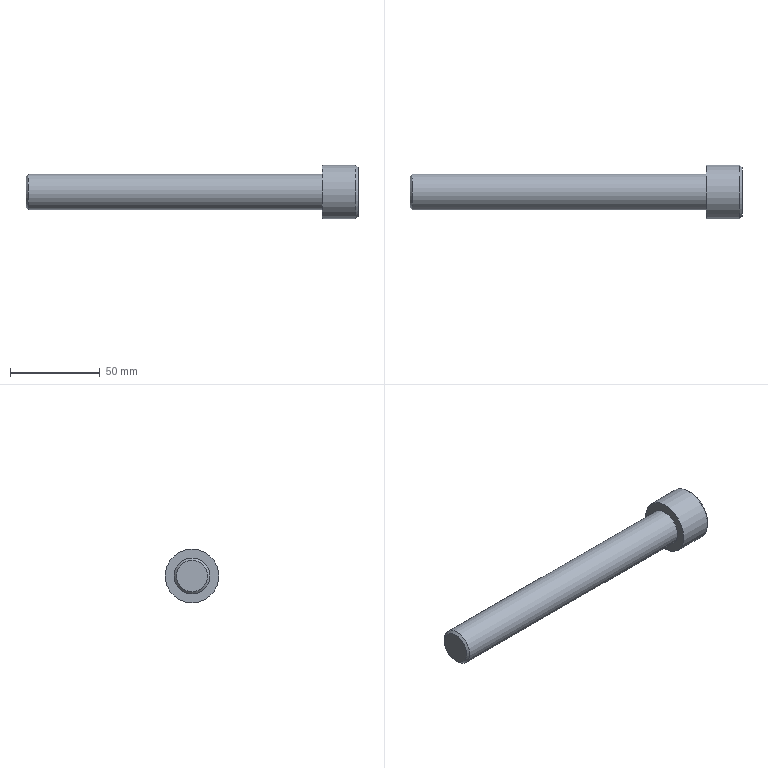Part | STEP file | solid 160 | 1 solid | 14 faces | box 185 x 30 x 30 mm | volume 63102 mm3 | plane 10 | cylinder 2 | cone 2 | commonest cylinder face diameters 20 x1 30 x1